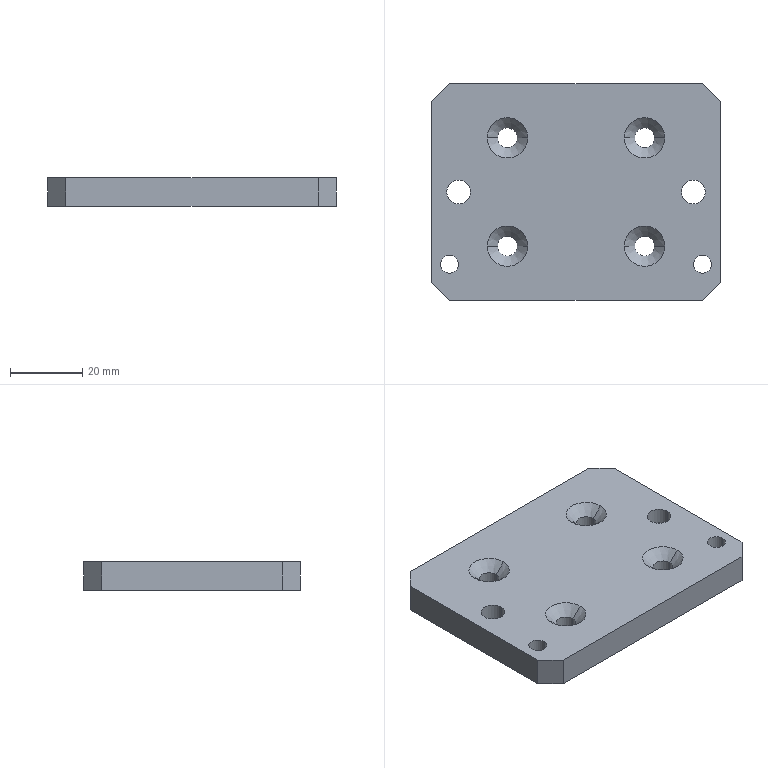Part | STEP file | Slider connection plate | 1 solid | 38 faces | box 80 x 60 x 8 mm | volume 35674 mm3 | cylinder 16 | cone 12 | plane 10 | commonest cylinder face diameters 5.5 x8 5 x4 6.6 x4